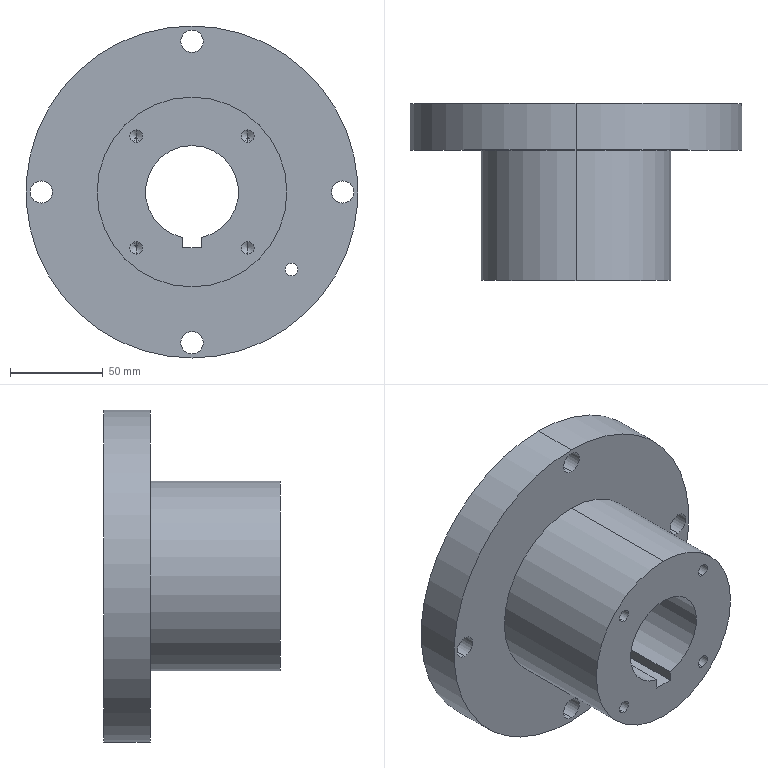Part | SolidWorks | features BaseBody 1 | 1 solid | 56 faces | box 178.5 x 95 x 178.5 mm | volume 847638 mm3 | cylinder 33 | cone 16 | plane 7 | commonest cylinder face diameters 6.8 x10 3.3 x8 12 x8 102 x2 143.5 x2 178.5 x2